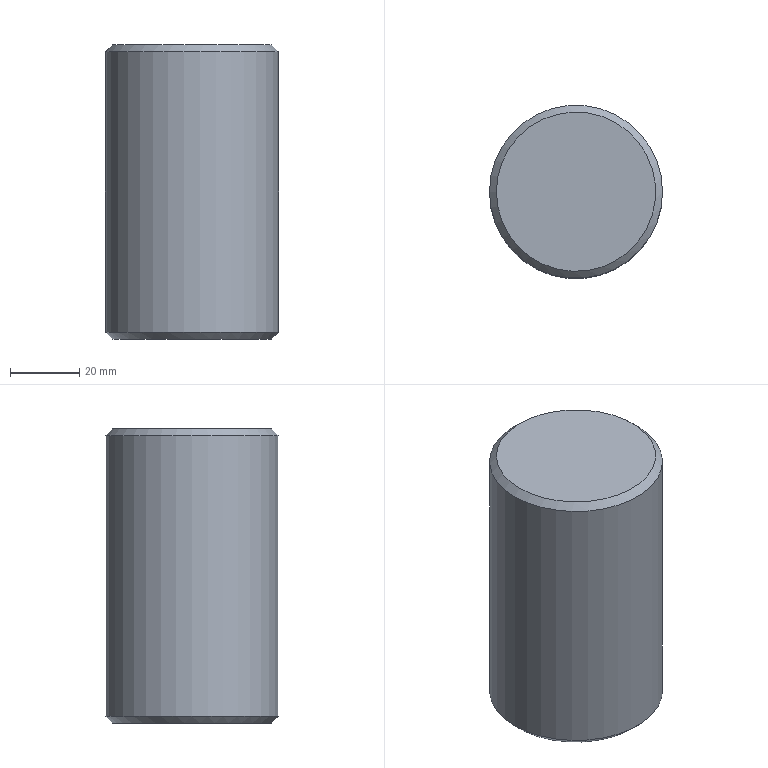Part | STEP file | 车灯-后视镜_id22_x_t | 1 solid | 9 faces | box 50 x 50 x 85 mm | volume 164490 mm3 | plane 3 | cylinder 3 | cone 3 | commonest cylinder face diameters 8.6 x1 10 x1 50 x1
STEP:
#1=CARTESIAN_POINT('',(87.,-75.,-285.5));
#2=VERTEX_POINT('',#1);
#3=CARTESIAN_POINT('',(110.,-75.,-285.5));
#4=DIRECTION('',(0.,0.,1.));
#5=DIRECTION('',(-1.,0.,0.));
#6=AXIS2_PLACEMENT_3D('',#3,#4,#5);
#7=CIRCLE('',#6,23.);
#8=EDGE_CURVE('',#2,#2,#7,.T.);
#9=ORIENTED_EDGE('',*,*,#8,.T.);
#10=EDGE_LOOP('',(#9));
#11=FACE_OUTER_BOUND('',#10,.T.);
#12=CARTESIAN_POINT('',(110.,-75.,-285.5));
#13=DIRECTION('',(0.,0.,1.));
#14=DIRECTION('',(-1.,0.,0.));
#15=AXIS2_PLACEMENT_3D('',#12,#13,#14);
#16=PLANE('',#15);
#17=ADVANCED_FACE('',(#11),#16,.T.);
#18=CARTESIAN_POINT('',(133.,-75.,-370.5));
#19=VERTEX_POINT('',#18);
#20=CARTESIAN_POINT('',(110.,-75.,-370.5));
#21=DIRECTION('',(0.,0.,-1.));
#22=DIRECTION('',(1.,0.,0.));
#23=AXIS2_PLACEMENT_3D('',#20,#21,#22);
#24=CIRCLE('',#23,23.);
#25=EDGE_CURVE('',#19,#19,#24,.T.);
#26=ORIENTED_EDGE('',*,*,#25,.T.);
#27=EDGE_LOOP('',(#26));
#28=FACE_BOUND('',#27,.T.);
#29=CARTESIAN_POINT('',(105.,-75.,-370.5));
#30=VERTEX_POINT('',#29);
#31=CARTESIAN_POINT('',(110.,-75.,-370.5));
#32=DIRECTION('',(0.,0.,1.));
#33=DIRECTION('',(-1.,0.,0.));
#34=AXIS2_PLACEMENT_3D('',#31,#32,#33);
#35=CIRCLE('',#34,5.);
#36=EDGE_CURVE('',#30,#30,#35,.T.);
#37=ORIENTED_EDGE('',*,*,#36,.T.);
#38=EDGE_LOOP('',(#37));
#39=FACE_BOUND('',#38,.T.);
#40=CARTESIAN_POINT('',(110.,-75.,-370.5));
#41=DIRECTION('',(0.,0.,-1.));
#42=DIRECTION('',(1.,0.,0.));
#43=AXIS2_PLACEMENT_3D('',#40,#41,#42);
#44=PLANE('',#43);
#45=ADVANCED_FACE('',(#28,#39),#44,.T.);
#46=CARTESIAN_POINT('',(85.,-75.,-287.5));
#47=VERTEX_POINT('',#46);
#48=CARTESIAN_POINT('',(110.,-75.,-287.5));
#49=DIRECTION('',(0.,0.,-1.));
#50=DIRECTION('',(-1.,0.,0.));
#51=AXIS2_PLACEMENT_3D('',#48,#49,#50);
#52=CIRCLE('',#51,25.);
#53=EDGE_CURVE('',#47,#47,#52,.T.);
#54=ORIENTED_EDGE('',*,*,#53,.T.);
#55=EDGE_LOOP('',(#54));
#56=FACE_BOUND('',#55,.T.);
#57=CARTESIAN_POINT('',(135.,-75.,-368.5));
#58=VERTEX_POINT('',#57);
#59=CARTESIAN_POINT('',(110.,-75.,-368.5));
#60=DIRECTION('',(0.,0.,1.));
#61=DIRECTION('',(1.,0.,0.));
#62=AXIS2_PLACEMENT_3D('',#59,#60,#61);
#63=CIRCLE('',#62,25.);
#64=EDGE_CURVE('',#58,#58,#63,.T.);
#65=ORIENTED_EDGE('',*,*,#64,.T.);
#66=EDGE_LOOP('',(#65));
#67=FACE_BOUND('',#66,.T.);
#68=CARTESIAN_POINT('',(110.,-75.,-330.5));
#69=DIRECTION('',(0.,0.,1.));
#70=DIRECTION('',(-1.,0.,0.));
#71=AXIS2_PLACEMENT_3D('',#68,#69,#70);
#72=CYLINDRICAL_SURFACE('',#71,25.);
#73=ADVANCED_FACE('',(#56,#67),#72,.T.);
#74=CARTESIAN_POINT('',(114.3,-75.,-347.5));
#75=VERTEX_POINT('',#74);
#76=CARTESIAN_POINT('',(110.,-75.,-347.5));
#77=DIRECTION('',(0.,0.,-1.));
#78=DIRECTION('',(1.,0.,0.));
#79=AXIS2_PLACEMENT_3D('',#76,#77,#78);
#80=CIRCLE('',#79,4.3);
#81=EDGE_CURVE('',#75,#75,#80,.T.);
#82=ORIENTED_EDGE('',*,*,#81,.F.);
#83=EDGE_LOOP('',(#82));
#84=FACE_BOUND('',#83,.T.);
#85=CARTESIAN_POINT('',(105.7,-75.,-350.5));
#86=VERTEX_POINT('',#85);
#87=CARTESIAN_POINT('',(110.,-75.,-350.5));
#88=DIRECTION('',(0.,0.,-1.));
#89=DIRECTION('',(-1.,0.,0.));
#90=AXIS2_PLACEMENT_3D('',#87,#88,#89);
#91=CIRCLE('',#90,4.3);
#92=EDGE_CURVE('',#86,#86,#91,.T.);
#93=ORIENTED_EDGE('',*,*,#92,.T.);
#94=EDGE_LOOP('',(#93));
#95=FACE_BOUND('',#94,.T.);
#96=CARTESIAN_POINT('',(110.,-75.,-350.5));
#97=DIRECTION('',(0.,0.,1.));
#98=DIRECTION('',(-1.,0.,0.));
#99=AXIS2_PLACEMENT_3D('',#96,#97,#98);
#100=CYLINDRICAL_SURFACE('',#99,4.3);
#101=ADVANCED_FACE('',(#84,#95),#100,.F.);
#102=ORIENTED_EDGE('',*,*,#81,.T.);
#103=EDGE_LOOP('',(#102));
#104=FACE_BOUND('',#103,.T.);
#105=CARTESIAN_POINT('',(110.,-75.,-344.916));
#106=VERTEX_POINT('',#105);
#107=VERTEX_LOOP('',#106);
#108=FACE_BOUND('',#107,.T.);
#109=CARTESIAN_POINT('',(110.,-75.,-344.916));
#110=DIRECTION('',(0.,0.,-1.));
#111=DIRECTION('',(1.,0.,0.));
#112=AXIS2_PLACEMENT_3D('',#109,#110,#111);
#113=CONICAL_SURFACE('',#112,0.,59.);
#114=ADVANCED_FACE('',(#104,#108),#113,.F.);
#115=ORIENTED_EDGE('',*,*,#92,.F.);
#116=EDGE_LOOP('',(#115));
#117=FACE_BOUND('',#116,.T.);
#118=CARTESIAN_POINT('',(115.,-75.,-350.5));
#119=VERTEX_POINT('',#118);
#120=CARTESIAN_POINT('',(110.,-75.,-350.5));
#121=DIRECTION('',(0.,0.,-1.));
#122=DIRECTION('',(1.,0.,0.));
#123=AXIS2_PLACEMENT_3D('',#120,#121,#122);
#124=CIRCLE('',#123,5.);
#125=EDGE_CURVE('',#119,#119,#124,.T.);
#126=ORIENTED_EDGE('',*,*,#125,.T.);
#127=EDGE_LOOP('',(#126));
#128=FACE_BOUND('',#127,.T.);
#129=CARTESIAN_POINT('',(110.,-75.,-350.5));
#130=DIRECTION('',(0.,0.,1.));
#131=DIRECTION('',(-1.,0.,0.));
#132=AXIS2_PLACEMENT_3D('',#129,#130,#131);
#133=PLANE('',#132);
#134=ADVANCED_FACE('',(#117,#128),#133,.F.);
#135=ORIENTED_EDGE('',*,*,#125,.F.);
#136=EDGE_LOOP('',(#135));
#137=FACE_BOUND('',#136,.T.);
#138=ORIENTED_EDGE('',*,*,#36,.F.);
#139=EDGE_LOOP('',(#138));
#140=FACE_BOUND('',#139,.T.);
#141=CARTESIAN_POINT('',(110.,-75.,-370.5));
#142=DIRECTION('',(0.,0.,1.));
#143=DIRECTION('',(-1.,0.,0.));
#144=AXIS2_PLACEMENT_3D('',#141,#142,#143);
#145=CYLINDRICAL_SURFACE('',#144,5.);
#146=ADVANCED_FACE('',(#137,#140),#145,.F.);
#147=ORIENTED_EDGE('',*,*,#25,.F.);
#148=EDGE_LOOP('',(#147));
#149=FACE_BOUND('',#148,.T.);
#150=ORIENTED_EDGE('',*,*,#64,.F.);
#151=EDGE_LOOP('',(#150));
#152=FACE_BOUND('',#151,.T.);
#153=CARTESIAN_POINT('',(110.,-75.,-368.5));
#154=DIRECTION('',(0.,0.,1.));
#155=DIRECTION('',(-1.,0.,0.));
#156=AXIS2_PLACEMENT_3D('',#153,#154,#155);
#157=CONICAL_SURFACE('',#156,25.,45.);
#158=ADVANCED_FACE('',(#149,#152),#157,.T.);
#159=ORIENTED_EDGE('',*,*,#8,.F.);
#160=EDGE_LOOP('',(#159));
#161=FACE_BOUND('',#160,.T.);
#162=ORIENTED_EDGE('',*,*,#53,.F.);
#163=EDGE_LOOP('',(#162));
#164=FACE_BOUND('',#163,.T.);
#165=CARTESIAN_POINT('',(110.,-75.,-287.5));
#166=DIRECTION('',(0.,0.,-1.));
#167=DIRECTION('',(1.,0.,0.));
#168=AXIS2_PLACEMENT_3D('',#165,#166,#167);
#169=CONICAL_SURFACE('',#168,25.,45.);
#170=ADVANCED_FACE('',(#161,#164),#169,.T.);
#171=CLOSED_SHELL('',(#17,#45,#73,#101,#114,#134,#146,#158,#170));
#172=MANIFOLD_SOLID_BREP('',#171);
#173=(LENGTH_UNIT()NAMED_UNIT(*)SI_UNIT(.MILLI.,.METRE.));
#174=UNCERTAINTY_MEASURE_WITH_UNIT(LENGTH_MEASURE(0.00002),#173,'','');
#175=(NAMED_UNIT(*)PLANE_ANGLE_UNIT()SI_UNIT($,.RADIAN.));
#176=PLANE_ANGLE_MEASURE_WITH_UNIT(PLANE_ANGLE_MEASURE(0.01745),#175);
#177=DIMENSIONAL_EXPONENTS(0.,0.,0.,0.,0.,0.,0.);
#178=(CONVERSION_BASED_UNIT('DEGREE',#176)NAMED_UNIT(#177)PLANE_ANGLE_UNIT());
#179=(NAMED_UNIT(*)SI_UNIT($,.STERADIAN.)SOLID_ANGLE_UNIT());
#180=(GEOMETRIC_REPRESENTATION_CONTEXT(3)GLOBAL_UNCERTAINTY_ASSIGNED_CONTEXT((#174))GLOBAL_UNIT_ASSIGNED_CONTEXT((#173,#178,#179))REPRESENTATION_CONTEXT('',''));
#181=ADVANCED_BREP_SHAPE_REPRESENTATION('',(#172),#180);